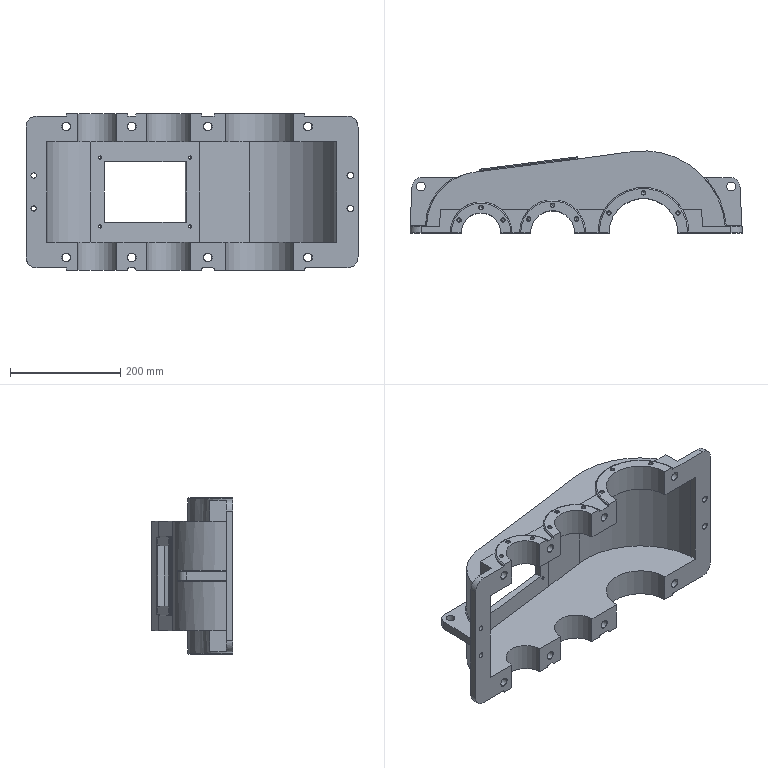Part | NX | 1 solid | 234 faces | box 603 x 149 x 284 mm | volume 3323600 mm3 | cylinder 77 | plane 75 | cone 67 | torus 10 | spline 5 | commonest cylinder face diameters 6.8 x18 4 x10 15 x8 28.5 x8 5 x4 40 x4